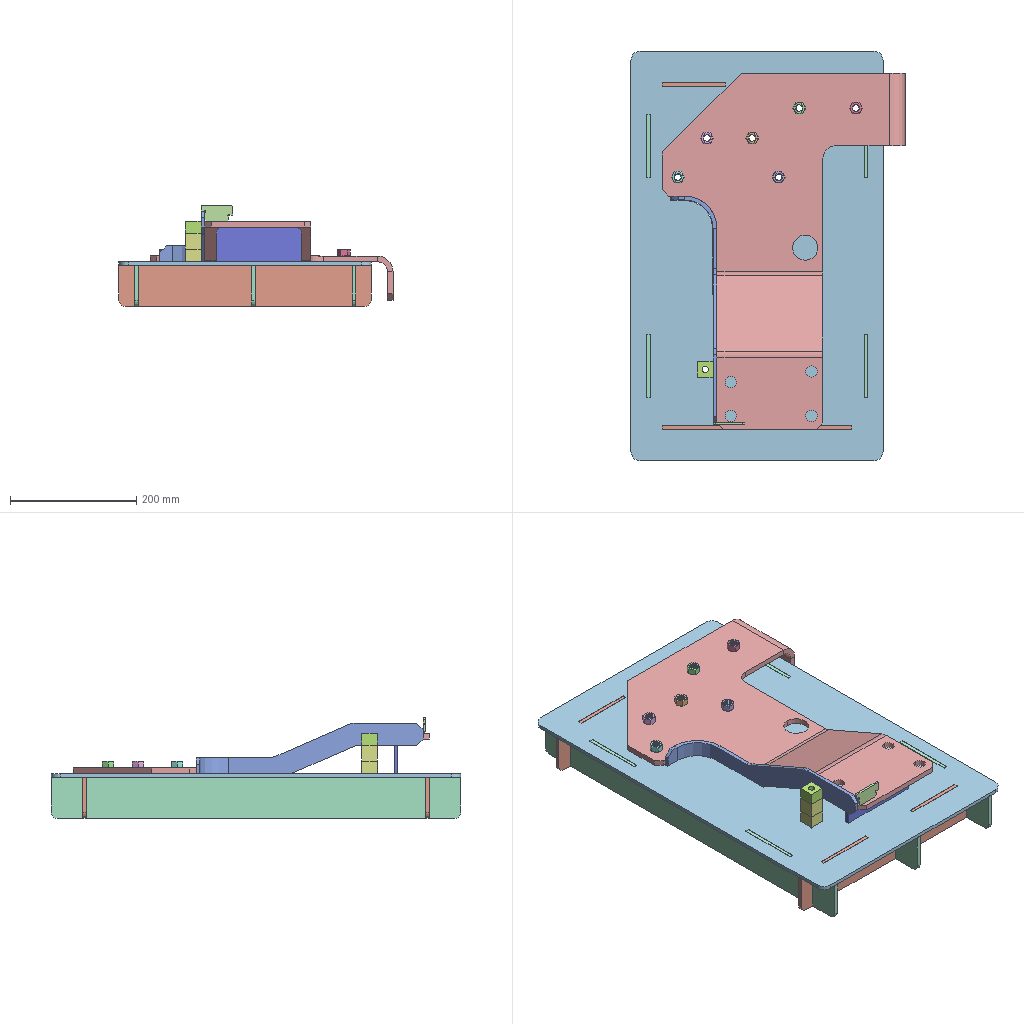Assembly | SolidWorks | 8 different items | 14 placed | box 435 x 650 x 160 mm
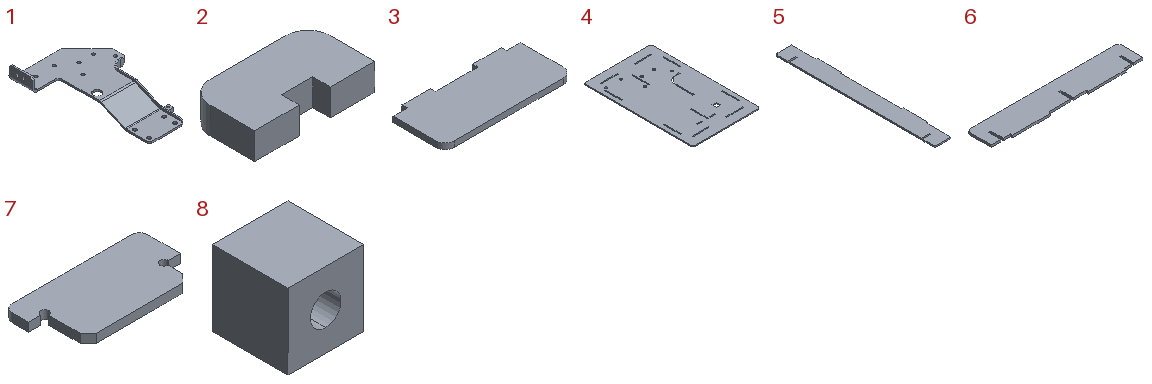Parts list (item | quantity | size | volume | features):
1 | x1 | 385 x 565 x 141 mm | 1220109 mm3 | features BaseBody 9, CosmeticWeldCutList 1
2 | x3 | 27 x 15 x 6 mm | 2198 mm3 | features FlatPattern 1, SMBaseFlange 1, SheetMetal 1
3 | x1 | 135 x 60.5 x 6 mm | 46272 mm3 | features FlatPattern 1, SMBaseFlange 1, SheetMetal 1
4 | x1 | 400 x 650 x 6 mm | 1502114 mm3 | features FlatPattern 1, SMBaseFlange 1, SheetMetal 1
5 | x3 | 70.5 x 650 x 6 mm | 257466 mm3 | features FlatPattern 1, SMBaseFlange 1, SheetMetal 1
6 | x2 | 400 x 70.5 x 6 mm | 158832 mm3 | features FlatPattern 1, SMBaseFlange 1, SheetMetal 1
7 | x1 | 50 x 25 x 3.2 mm | 3426 mm3 | features FlatPattern 1, SMBaseFlange 1, SheetMetal 1
8 | x2 | 25 x 25 x 25 mm | 13582 mm3 | features Extrusion 1, HoleWzd 1
Mates (type | each side: item.copy, entity, surface, feature):
InPlace | 1.1 face plane | 4.1 plane
Coincident | 1.1 face plane PN_0001-1-solid1 | 8.1 face plane Boss-Extrude1 | 3 times
InPlace | 2.1 plane | assembly plane
Coincident | 4.1 face plane Base-Flange1 | 2.2 face plane Base-Flange1 | 2 times
DistanceDim | 2.2 face plane Base-Flange1 | 4.1 face plane Base-Flange1
InPlace | 5.1 plane | assembly plane
InPlace | 6.1 plane | assembly plane
InPlace | 3.1 plane | assembly plane
InPlace | 1.1 face plane | 7.1 plane